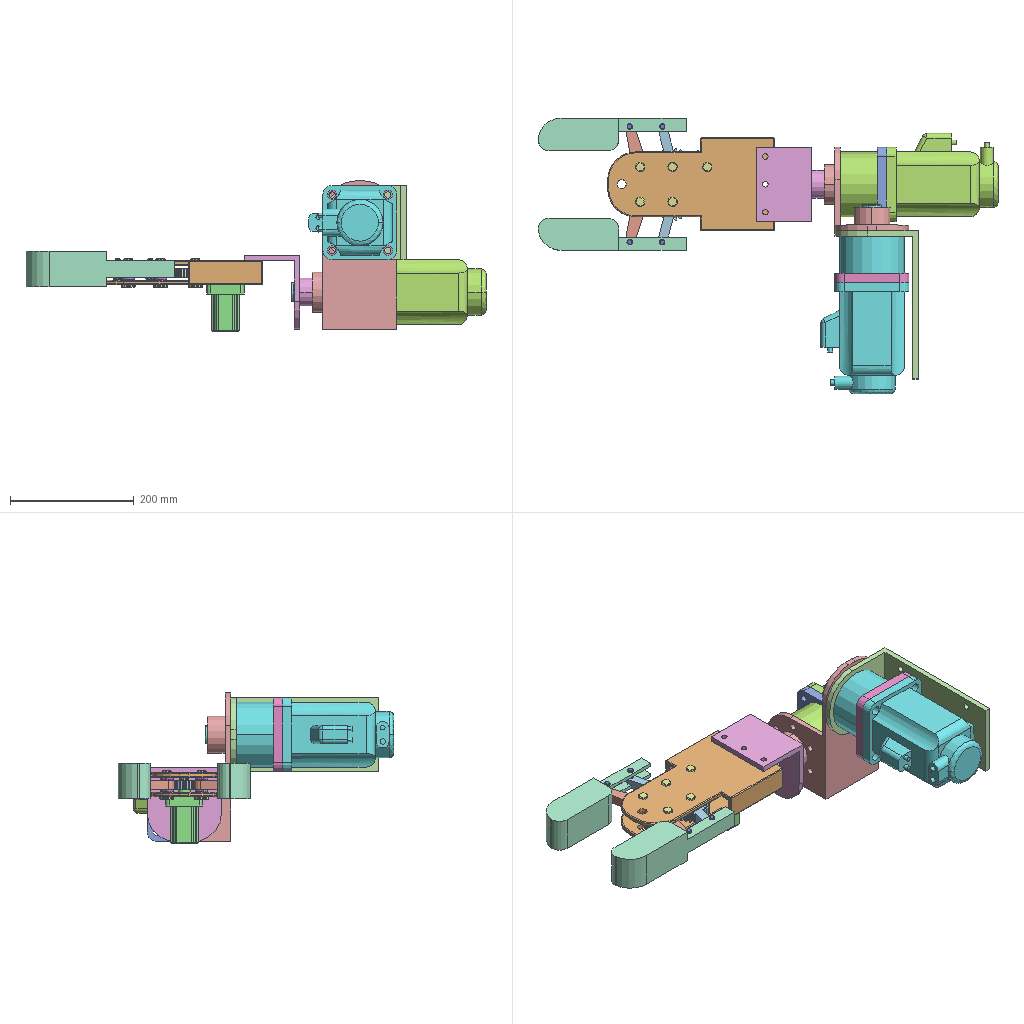Assembly | SolidWorks | 27 different items | 47 placed | box 744 x 446 x 243 mm
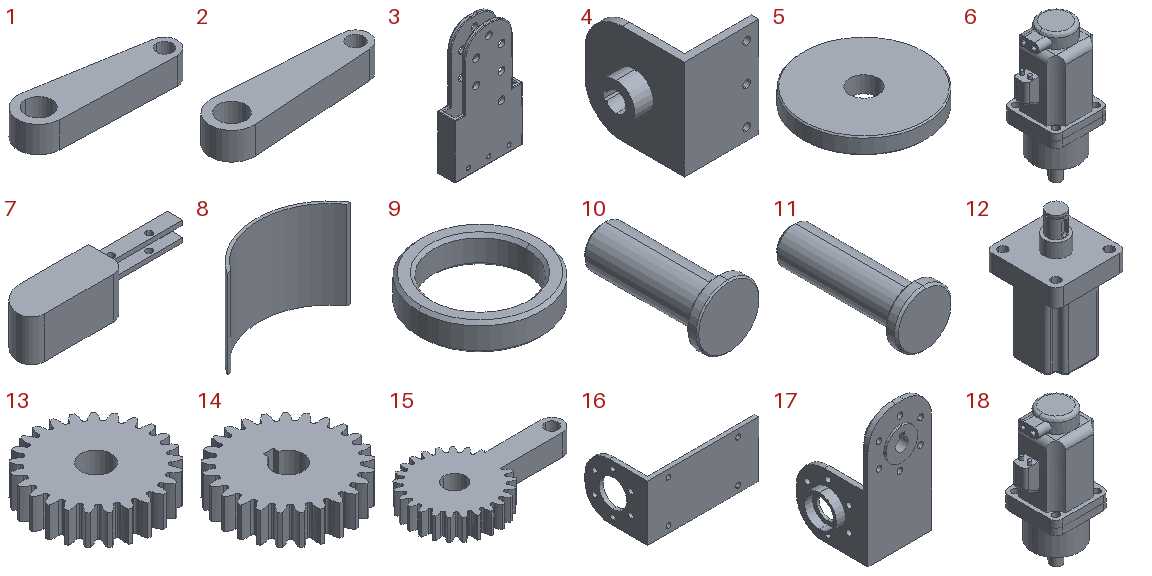Parts list (item | name | quantity | size | volume | features):
1 | - | x1 | 84.765 x 26.042 x 15 mm | 20344 mm3 | features BaseBody 1
2 | - | x2 | 87 x 24 x 15 mm | 20884 mm3 | features Extrusion 1
3 | - | x1 | 150 x 39 x 270 mm | 515829 mm3 | features ICE 2, 3DProfileFeature 1, BaseBody 1, HoleWzd 1
4 | - | x1 | 112.5 x 120 x 120 mm | 228143 mm3 | features ICE 2, BaseBody 1
5 | - | x2 | 30 x 30 x 4 mm | 2665 mm3 | features Chamfer 1, Extrusion 1
6 | - | x1 | 142.5 x 120 x 309 mm | 2592424 mm3 | features BaseBody 2, 3DProfileFeature 1, HoleWzd 1, ICE 1
7 | - | x2 | 239.768 x 52.5 x 57 mm | 402739 mm3 | features BaseBody 1, ICE 1
8 | - | x1 | 80 x 21.467 x 57 mm | 10404 mm3 | features Extrusion 1
9 | - | x10 | 20 x 20 x 4.5 mm | 591.012 mm3 | features Chamfer 1, Extrusion 1
10 | - | x5 | 23 x 46 x 23 mm | 9044 mm3 | features Chamfer 2, Extrusion 1, ICE 1
11 | - | x4 | 14 x 33 x 14 mm | 2347 mm3 | features Chamfer 2, Extrusion 1, ICE 1
12 | - | x1 | 60 x 60 x 105 mm | 154768 mm3 | features ICE 5, BaseBody 1
13 | - | x1 | 60.71 x 60.601 x 15 mm | 34143 mm3 | features BaseBody 1
14 | - | x1 | 60.71 x 60.601 x 15 mm | 33960 mm3 | features BaseBody 1, ICE 1
15 | - | x2 | 105.355 x 60.601 x 15 mm | 43506 mm3 | features BaseBody 1
16 | - | x1 | 240 x 135 x 120 mm | 351393 mm3 | features ICE 3, BaseBody 1
17 | - | x1 | 137 x 139 x 240 mm | 432649 mm3 | features ICE 6, BaseBody 1, CirPattern 1
18 | - | x1 | 142.5 x 120 x 301.5 mm | 2581853 mm3 | features ICE 3, BaseBody 2, 3DProfileFeature 1, HoleWzd 1
19 | GB894.1-86 Shaft Retaining Ring A Type15 | x1 | - | - | -
20 | GB/T1096-1979 Parallel Key A Type5×13 | x1 | - | - | -
21 | GB/T276-94 Deep Groove Ball Bearing6006-2RZ | x1 | - | - | -
22 | GB/T5781-2000 Hex Head Bolt Fully Threaded C Grade M6×25 | x1 | - | - | -
23 | GB/T6183.2-2000 Nylon Insert Hex Flange Lock Nut M8 | x1 | - | - | -
24 | GB/T70.1-2000 Socket Head Cap Screw M10×30 | x1 | - | - | -
25 | GB/T70.1-2000 Socket Head Cap Screw M10×50 | x1 | - | - | -
26 | GB/T70.1-2000 Socket Head Cap Screw M6×20 | x1 | - | - | -
27 | GB/T70.1-2000 Socket Head Cap Screw M8×35 | x1 | - | - | -
Mates (type | each side: item.copy, entity, surface, feature):
Coincident | 17.1 plane | assembly plane | 3 times
Concentric | 17.1 face cylinder Input1 | 6.1 face cylinder Input2
Parallel | 17.1 face plane Input1 | 6.1 face plane Input2
Coincident | 17.1 face plane Input1 | 6.1 face plane Input2
Concentric | 6.1 face cylinder Input2 | 4.1 face cylinder Input1
Parallel | 6.1 face plane Input2 | 4.1 face plane Input1
Concentric | 6.1 face cylinder M6 Tapped Hole1 | 5.1 face cylinder Boss-Extrude1
Coincident | 4.1 face plane Input1 | 5.1 face plane Boss-Extrude1
Concentric | 4.1 face cylinder Boss-Extrude1 | 3.1 face cylinder Cut-Extrude2 | 2 times
Coincident | 4.1 face plane Input1 | 3.1 face plane Input1
Concentric | 3.1 face cylinder Input1 | 12.1 face cylinder Boss-Extrude2
Coincident | 3.1 face plane Input1 | 12.1 face plane Input1
Concentric | 12.1 face cylinder Boss-Extrude3 | 14.1 face cylinder Input1
Width | 14.1 face plane Input1 | 14.1 face plane Input1 | 3.1 face plane Input1 | 3.1 face plane Input1
Parallel | 12.1 face plane Cut-Extrude1 | 14.1 face plane Cut-Extrude1
Parallel | 3.1 face plane Input1 | 14.1 face plane Cut-Extrude1
Concentric | 3.1 face cylinder Input1 | 10.1 face cylinder Boss-Extrude2
Coincident | 3.1 face plane Input1 | 10.1 face plane Boss-Extrude1
Concentric | 10.1 face cylinder Boss-Extrude2 | 9.1 face cylinder Boss-Extrude1
Concentric | 10.1 face cylinder Boss-Extrude2 | 9.2 face cylinder Boss-Extrude1
Concentric | 3.1 face cylinder Input1 | 15.1 face cylinder Input1
Concentric | 3.1 face cylinder Input1 | 10.2 face cylinder Boss-Extrude2
Coincident | 3.1 face plane Input1 | 10.2 face plane Boss-Extrude1
Concentric | 10.2 face cylinder Boss-Extrude2 | 9.3 face cylinder Boss-Extrude1
Coincident | 15.1 face plane Input1 | 9.3 face plane Boss-Extrude1
Concentric | 10.2 face cylinder Boss-Extrude2 | 9.4 face cylinder Boss-Extrude1
Coincident | 15.1 face plane Input1 | 9.4 face plane Boss-Extrude1
Concentric | 3.1 face cylinder Input1 | 10.3 face cylinder Boss-Extrude2
Coincident | 3.1 face plane Input1 | 10.3 face plane Boss-Extrude1
Concentric | 10.3 face cylinder Boss-Extrude2 | 9.5 face cylinder Boss-Extrude1
Concentric | 10.3 face cylinder Boss-Extrude2 | 9.6 face cylinder Boss-Extrude1
Concentric | 15.1 face cylinder Input1 | 7.1 face cylinder Input1
Concentric | 10.3 face cylinder Boss-Extrude2 | 2.1 face cylinder Boss-Extrude1
Coincident | 15.1 face plane Input1 | 2.1 face plane Boss-Extrude1
Coincident | 9.5 face plane Boss-Extrude1 | 2.1 face plane Boss-Extrude1
Coincident | 9.6 face plane Boss-Extrude1 | 2.1 face plane Boss-Extrude1
Concentric | 7.1 face cylinder Input1 | 2.1 face cylinder Boss-Extrude1
Concentric | 7.1 face cylinder Input1 | 11.1 face cylinder Boss-Extrude2
Coincident | 7.1 face plane Input1 | 11.1 face plane Boss-Extrude1
Concentric | 7.1 face cylinder Input1 | 11.2 face cylinder Boss-Extrude2
Coincident | 7.1 face plane Input1 | 11.2 face plane Boss-Extrude1
Concentric | 17.1 face cylinder Input1 | 16.1 face cylinder Input1
Parallel | 17.1 face plane Input1 | 16.1 face plane Input1
Coincident | 17.1 face plane Input1 | 16.1 face plane Input1
Concentric | 17.1 face cylinder Input1 | 18.1 face cylinder Input3
Parallel | 16.1 face plane Input1 | 18.1 face plane Input1
Coincident | 16.1 face plane Input1 | 18.1 face plane Input3
Concentric | 18.1 face cylinder M6 Tapped Hole1 | 5.2 face cylinder Boss-Extrude1
Coincident | 17.1 face plane Input1 | 5.2 face plane Boss-Extrude1
Concentric | 10.1 face cylinder Boss-Extrude2 | 13.1 face cylinder Input1
Coincident | 14.1 face plane Input1 | 13.1 face plane Input1
Coincident | 15.1 face plane Input1 | 13.1 face plane Input1
Concentric | 10.4 face cylinder Boss-Extrude2 | 15.2 face cylinder Input1
Coincident | 15.1 face plane Input1 | 15.2 face plane Input1
Coincident | 2.2 face plane Boss-Extrude1 | 7.2 face plane Input1